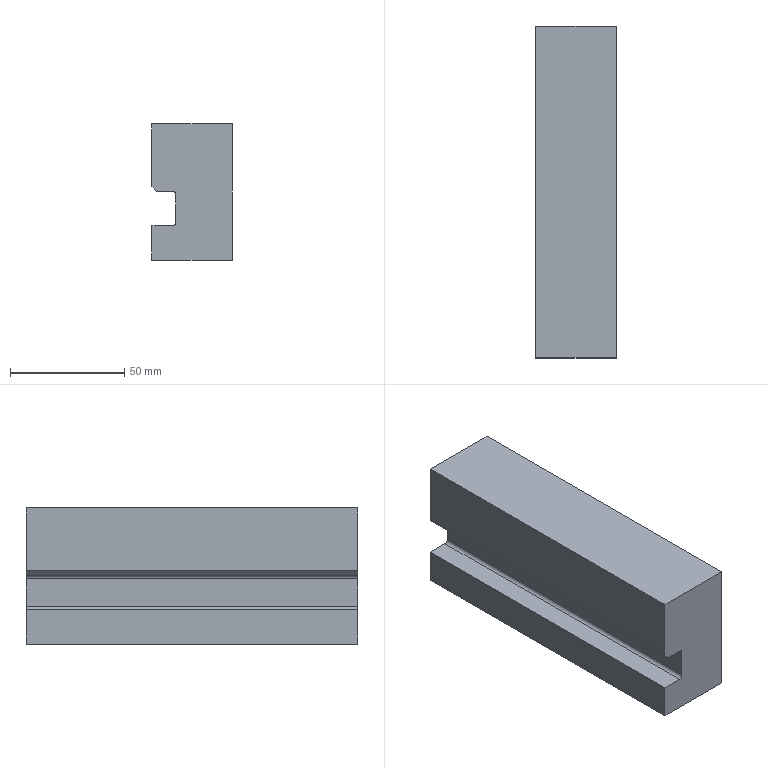Part | SolidWorks | features BaseBody 1 | 1 solid | 43 faces | box 35 x 145 x 59.5 mm | volume 272412 mm3 | plane 25 | cylinder 10 | cone 8 | commonest cylinder face diameters 8.5 x8 3 x2
STEP:
#1=CARTESIAN_POINT('',(214.249,235.,-60.));
#2=VERTEX_POINT('',#1);
#3=CARTESIAN_POINT('',(222.749,235.,-60.));
#4=VERTEX_POINT('',#3);
#5=CARTESIAN_POINT('',(218.499,235.,-60.));
#6=DIRECTION('',(0.,0.,-1.));
#7=DIRECTION('',(-1.,0.,0.));
#8=AXIS2_PLACEMENT_3D('',#5,#6,#7);
#9=CIRCLE('',#8,4.25);
#10=EDGE_CURVE('',#2,#4,#9,.T.);
#11=ORIENTED_EDGE('',*,*,#10,.T.);
#12=CARTESIAN_POINT('',(222.749,235.,-32.));
#13=VERTEX_POINT('',#12);
#14=CARTESIAN_POINT('',(222.749,235.,-60.));
#15=DIRECTION('',(0.,0.,1.));
#16=VECTOR('',#15,1000.);
#17=LINE('',#14,#16);
#18=EDGE_CURVE('',#4,#13,#17,.T.);
#19=ORIENTED_EDGE('',*,*,#18,.T.);
#20=CARTESIAN_POINT('',(214.249,235.,-32.));
#21=VERTEX_POINT('',#20);
#22=CARTESIAN_POINT('',(218.499,235.,-32.));
#23=DIRECTION('',(0.,0.,-1.));
#24=DIRECTION('',(-1.,0.,0.));
#25=AXIS2_PLACEMENT_3D('',#22,#23,#24);
#26=CIRCLE('',#25,4.25);
#27=EDGE_CURVE('',#21,#13,#26,.T.);
#28=ORIENTED_EDGE('',*,*,#27,.F.);
#29=CARTESIAN_POINT('',(214.249,235.,-60.));
#30=DIRECTION('',(0.,0.,1.));
#31=VECTOR('',#30,1000.);
#32=LINE('',#29,#31);
#33=EDGE_CURVE('',#2,#21,#32,.T.);
#34=ORIENTED_EDGE('',*,*,#33,.F.);
#35=EDGE_LOOP('',(#11,#19,#28,#34));
#36=FACE_OUTER_BOUND('',#35,.T.);
#37=CARTESIAN_POINT('',(218.499,235.,-60.));
#38=DIRECTION('',(0.,0.,1.));
#39=DIRECTION('',(-1.,0.,0.));
#40=AXIS2_PLACEMENT_3D('',#37,#38,#39);
#41=CYLINDRICAL_SURFACE('',#40,4.25);
#42=ADVANCED_FACE('',(#36),#41,.F.);
#43=CARTESIAN_POINT('',(218.499,235.,-29.446));
#44=VERTEX_POINT('',#43);
#45=CARTESIAN_POINT('',(222.749,235.,-32.));
#46=DIRECTION('',(0.8572,0.,-0.515));
#47=VECTOR('',#46,1000.);
#48=LINE('',#45,#47);
#49=EDGE_CURVE('',#44,#13,#48,.T.);
#50=ORIENTED_EDGE('',*,*,#49,.F.);
#51=CARTESIAN_POINT('',(214.249,235.,-32.));
#52=DIRECTION('',(-0.8572,0.,-0.515));
#53=VECTOR('',#52,1000.);
#54=LINE('',#51,#53);
#55=EDGE_CURVE('',#44,#21,#54,.T.);
#56=ORIENTED_EDGE('',*,*,#55,.T.);
#57=ORIENTED_EDGE('',*,*,#27,.T.);
#58=EDGE_LOOP('',(#50,#56,#57));
#59=FACE_OUTER_BOUND('',#58,.T.);
#60=CARTESIAN_POINT('',(218.499,235.,-32.));
#61=DIRECTION('',(0.,0.,-1.));
#62=DIRECTION('',(1.,0.,0.));
#63=AXIS2_PLACEMENT_3D('',#60,#61,#62);
#64=CONICAL_SURFACE('',#63,4.25,1.03);
#65=ADVANCED_FACE('',(#59),#64,.F.);
#66=CARTESIAN_POINT('',(214.249,270.,-60.));
#67=VERTEX_POINT('',#66);
#68=CARTESIAN_POINT('',(222.749,270.,-60.));
#69=VERTEX_POINT('',#68);
#70=CARTESIAN_POINT('',(218.499,270.,-60.));
#71=DIRECTION('',(0.,0.,-1.));
#72=DIRECTION('',(-1.,0.,0.));
#73=AXIS2_PLACEMENT_3D('',#70,#71,#72);
#74=CIRCLE('',#73,4.25);
#75=EDGE_CURVE('',#67,#69,#74,.T.);
#76=ORIENTED_EDGE('',*,*,#75,.T.);
#77=CARTESIAN_POINT('',(222.749,270.,-32.));
#78=VERTEX_POINT('',#77);
#79=CARTESIAN_POINT('',(222.749,270.,-60.));
#80=DIRECTION('',(0.,0.,1.));
#81=VECTOR('',#80,1000.);
#82=LINE('',#79,#81);
#83=EDGE_CURVE('',#69,#78,#82,.T.);
#84=ORIENTED_EDGE('',*,*,#83,.T.);
#85=CARTESIAN_POINT('',(214.249,270.,-32.));
#86=VERTEX_POINT('',#85);
#87=CARTESIAN_POINT('',(218.499,270.,-32.));
#88=DIRECTION('',(0.,0.,-1.));
#89=DIRECTION('',(-1.,0.,0.));
#90=AXIS2_PLACEMENT_3D('',#87,#88,#89);
#91=CIRCLE('',#90,4.25);
#92=EDGE_CURVE('',#86,#78,#91,.T.);
#93=ORIENTED_EDGE('',*,*,#92,.F.);
#94=CARTESIAN_POINT('',(214.249,270.,-60.));
#95=DIRECTION('',(0.,0.,1.));
#96=VECTOR('',#95,1000.);
#97=LINE('',#94,#96);
#98=EDGE_CURVE('',#67,#86,#97,.T.);
#99=ORIENTED_EDGE('',*,*,#98,.F.);
#100=EDGE_LOOP('',(#76,#84,#93,#99));
#101=FACE_OUTER_BOUND('',#100,.T.);
#102=CARTESIAN_POINT('',(218.499,270.,-60.));
#103=DIRECTION('',(0.,0.,1.));
#104=DIRECTION('',(-1.,0.,0.));
#105=AXIS2_PLACEMENT_3D('',#102,#103,#104);
#106=CYLINDRICAL_SURFACE('',#105,4.25);
#107=ADVANCED_FACE('',(#101),#106,.F.);
#108=CARTESIAN_POINT('',(218.499,270.,-29.446));
#109=VERTEX_POINT('',#108);
#110=CARTESIAN_POINT('',(222.749,270.,-32.));
#111=DIRECTION('',(0.8572,0.,-0.515));
#112=VECTOR('',#111,1000.);
#113=LINE('',#110,#112);
#114=EDGE_CURVE('',#109,#78,#113,.T.);
#115=ORIENTED_EDGE('',*,*,#114,.F.);
#116=CARTESIAN_POINT('',(214.249,270.,-32.));
#117=DIRECTION('',(-0.8572,0.,-0.515));
#118=VECTOR('',#117,1000.);
#119=LINE('',#116,#118);
#120=EDGE_CURVE('',#109,#86,#119,.T.);
#121=ORIENTED_EDGE('',*,*,#120,.T.);
#122=ORIENTED_EDGE('',*,*,#92,.T.);
#123=EDGE_LOOP('',(#115,#121,#122));
#124=FACE_OUTER_BOUND('',#123,.T.);
#125=CARTESIAN_POINT('',(218.499,270.,-32.));
#126=DIRECTION('',(0.,0.,-1.));
#127=DIRECTION('',(1.,0.,0.));
#128=AXIS2_PLACEMENT_3D('',#125,#126,#127);
#129=CONICAL_SURFACE('',#128,4.25,1.03);
#130=ADVANCED_FACE('',(#124),#129,.F.);
#131=CARTESIAN_POINT('',(214.249,300.,-60.));
#132=VERTEX_POINT('',#131);
#133=CARTESIAN_POINT('',(222.749,300.,-60.));
#134=VERTEX_POINT('',#133);
#135=CARTESIAN_POINT('',(218.499,300.,-60.));
#136=DIRECTION('',(0.,0.,-1.));
#137=DIRECTION('',(-1.,0.,0.));
#138=AXIS2_PLACEMENT_3D('',#135,#136,#137);
#139=CIRCLE('',#138,4.25);
#140=EDGE_CURVE('',#132,#134,#139,.T.);
#141=ORIENTED_EDGE('',*,*,#140,.T.);
#142=CARTESIAN_POINT('',(222.749,300.,-32.));
#143=VERTEX_POINT('',#142);
#144=CARTESIAN_POINT('',(222.749,300.,-60.));
#145=DIRECTION('',(0.,0.,1.));
#146=VECTOR('',#145,1000.);
#147=LINE('',#144,#146);
#148=EDGE_CURVE('',#134,#143,#147,.T.);
#149=ORIENTED_EDGE('',*,*,#148,.T.);
#150=CARTESIAN_POINT('',(214.249,300.,-32.));
#151=VERTEX_POINT('',#150);
#152=CARTESIAN_POINT('',(218.499,300.,-32.));
#153=DIRECTION('',(0.,0.,-1.));
#154=DIRECTION('',(-1.,0.,0.));
#155=AXIS2_PLACEMENT_3D('',#152,#153,#154);
#156=CIRCLE('',#155,4.25);
#157=EDGE_CURVE('',#151,#143,#156,.T.);
#158=ORIENTED_EDGE('',*,*,#157,.F.);
#159=CARTESIAN_POINT('',(214.249,300.,-60.));
#160=DIRECTION('',(0.,0.,1.));
#161=VECTOR('',#160,1000.);
#162=LINE('',#159,#161);
#163=EDGE_CURVE('',#132,#151,#162,.T.);
#164=ORIENTED_EDGE('',*,*,#163,.F.);
#165=EDGE_LOOP('',(#141,#149,#158,#164));
#166=FACE_OUTER_BOUND('',#165,.T.);
#167=CARTESIAN_POINT('',(218.499,300.,-60.));
#168=DIRECTION('',(0.,0.,1.));
#169=DIRECTION('',(-1.,0.,0.));
#170=AXIS2_PLACEMENT_3D('',#167,#168,#169);
#171=CYLINDRICAL_SURFACE('',#170,4.25);
#172=ADVANCED_FACE('',(#166),#171,.F.);
#173=CARTESIAN_POINT('',(218.499,300.,-29.446));
#174=VERTEX_POINT('',#173);
#175=CARTESIAN_POINT('',(222.749,300.,-32.));
#176=DIRECTION('',(0.8572,0.,-0.515));
#177=VECTOR('',#176,1000.);
#178=LINE('',#175,#177);
#179=EDGE_CURVE('',#174,#143,#178,.T.);
#180=ORIENTED_EDGE('',*,*,#179,.F.);
#181=CARTESIAN_POINT('',(214.249,300.,-32.));
#182=DIRECTION('',(-0.8572,0.,-0.515));
#183=VECTOR('',#182,1000.);
#184=LINE('',#181,#183);
#185=EDGE_CURVE('',#174,#151,#184,.T.);
#186=ORIENTED_EDGE('',*,*,#185,.T.);
#187=ORIENTED_EDGE('',*,*,#157,.T.);
#188=EDGE_LOOP('',(#180,#186,#187));
#189=FACE_OUTER_BOUND('',#188,.T.);
#190=CARTESIAN_POINT('',(218.499,300.,-32.));
#191=DIRECTION('',(0.,0.,-1.));
#192=DIRECTION('',(1.,0.,0.));
#193=AXIS2_PLACEMENT_3D('',#190,#191,#192);
#194=CONICAL_SURFACE('',#193,4.25,1.03);
#195=ADVANCED_FACE('',(#189),#194,.F.);
#196=CARTESIAN_POINT('',(214.249,335.,-60.));
#197=VERTEX_POINT('',#196);
#198=CARTESIAN_POINT('',(222.749,335.,-60.));
#199=VERTEX_POINT('',#198);
#200=CARTESIAN_POINT('',(218.499,335.,-60.));
#201=DIRECTION('',(0.,0.,-1.));
#202=DIRECTION('',(-1.,0.,0.));
#203=AXIS2_PLACEMENT_3D('',#200,#201,#202);
#204=CIRCLE('',#203,4.25);
#205=EDGE_CURVE('',#197,#199,#204,.T.);
#206=ORIENTED_EDGE('',*,*,#205,.T.);
#207=CARTESIAN_POINT('',(222.749,335.,-32.));
#208=VERTEX_POINT('',#207);
#209=CARTESIAN_POINT('',(222.749,335.,-60.));
#210=DIRECTION('',(0.,0.,1.));
#211=VECTOR('',#210,1000.);
#212=LINE('',#209,#211);
#213=EDGE_CURVE('',#199,#208,#212,.T.);
#214=ORIENTED_EDGE('',*,*,#213,.T.);
#215=CARTESIAN_POINT('',(214.249,335.,-32.));
#216=VERTEX_POINT('',#215);
#217=CARTESIAN_POINT('',(218.499,335.,-32.));
#218=DIRECTION('',(0.,0.,-1.));
#219=DIRECTION('',(-1.,0.,0.));
#220=AXIS2_PLACEMENT_3D('',#217,#218,#219);
#221=CIRCLE('',#220,4.25);
#222=EDGE_CURVE('',#216,#208,#221,.T.);
#223=ORIENTED_EDGE('',*,*,#222,.F.);
#224=CARTESIAN_POINT('',(214.249,335.,-60.));
#225=DIRECTION('',(0.,0.,1.));
#226=VECTOR('',#225,1000.);
#227=LINE('',#224,#226);
#228=EDGE_CURVE('',#197,#216,#227,.T.);
#229=ORIENTED_EDGE('',*,*,#228,.F.);
#230=EDGE_LOOP('',(#206,#214,#223,#229));
#231=FACE_OUTER_BOUND('',#230,.T.);
#232=CARTESIAN_POINT('',(218.499,335.,-60.));
#233=DIRECTION('',(0.,0.,1.));
#234=DIRECTION('',(-1.,0.,0.));
#235=AXIS2_PLACEMENT_3D('',#232,#233,#234);
#236=CYLINDRICAL_SURFACE('',#235,4.25);
#237=ADVANCED_FACE('',(#231),#236,.F.);
#238=CARTESIAN_POINT('',(218.499,335.,-29.446));
#239=VERTEX_POINT('',#238);
#240=CARTESIAN_POINT('',(222.749,335.,-32.));
#241=DIRECTION('',(0.8572,0.,-0.515));
#242=VECTOR('',#241,1000.);
#243=LINE('',#240,#242);
#244=EDGE_CURVE('',#239,#208,#243,.T.);
#245=ORIENTED_EDGE('',*,*,#244,.F.);
#246=CARTESIAN_POINT('',(214.249,335.,-32.));
#247=DIRECTION('',(-0.8572,0.,-0.515));
#248=VECTOR('',#247,1000.);
#249=LINE('',#246,#248);
#250=EDGE_CURVE('',#239,#216,#249,.T.);
#251=ORIENTED_EDGE('',*,*,#250,.T.);
#252=ORIENTED_EDGE('',*,*,#222,.T.);
#253=EDGE_LOOP('',(#245,#251,#252));
#254=FACE_OUTER_BOUND('',#253,.T.);
#255=CARTESIAN_POINT('',(218.499,335.,-32.));
#256=DIRECTION('',(0.,0.,-1.));
#257=DIRECTION('',(1.,0.,0.));
#258=AXIS2_PLACEMENT_3D('',#255,#256,#257);
#259=CONICAL_SURFACE('',#258,4.25,1.03);
#260=ADVANCED_FACE('',(#254),#259,.F.);
#261=ORIENTED_EDGE('',*,*,#10,.F.);
#262=CARTESIAN_POINT('',(218.499,235.,-60.));
#263=DIRECTION('',(0.,0.,-1.));
#264=DIRECTION('',(-1.,0.,0.));
#265=AXIS2_PLACEMENT_3D('',#262,#263,#264);
#266=CIRCLE('',#265,4.25);
#267=EDGE_CURVE('',#4,#2,#266,.T.);
#268=ORIENTED_EDGE('',*,*,#267,.F.);
#269=EDGE_LOOP('',(#261,#268));
#270=FACE_BOUND('',#269,.T.);
#271=ORIENTED_EDGE('',*,*,#75,.F.);
#272=CARTESIAN_POINT('',(218.499,270.,-60.));
#273=DIRECTION('',(0.,0.,-1.));
#274=DIRECTION('',(-1.,0.,0.));
#275=AXIS2_PLACEMENT_3D('',#272,#273,#274);
#276=CIRCLE('',#275,4.25);
#277=EDGE_CURVE('',#69,#67,#276,.T.);
#278=ORIENTED_EDGE('',*,*,#277,.F.);
#279=EDGE_LOOP('',(#271,#278));
#280=FACE_BOUND('',#279,.T.);
#281=ORIENTED_EDGE('',*,*,#140,.F.);
#282=CARTESIAN_POINT('',(218.499,300.,-60.));
#283=DIRECTION('',(0.,0.,-1.));
#284=DIRECTION('',(-1.,0.,0.));
#285=AXIS2_PLACEMENT_3D('',#282,#283,#284);
#286=CIRCLE('',#285,4.25);
#287=EDGE_CURVE('',#134,#132,#286,.T.);
#288=ORIENTED_EDGE('',*,*,#287,.F.);
#289=EDGE_LOOP('',(#281,#288));
#290=FACE_BOUND('',#289,.T.);
#291=ORIENTED_EDGE('',*,*,#205,.F.);
#292=CARTESIAN_POINT('',(218.499,335.,-60.));
#293=DIRECTION('',(0.,0.,-1.));
#294=DIRECTION('',(-1.,0.,0.));
#295=AXIS2_PLACEMENT_3D('',#292,#293,#294);
#296=CIRCLE('',#295,4.25);
#297=EDGE_CURVE('',#199,#197,#296,.T.);
#298=ORIENTED_EDGE('',*,*,#297,.F.);
#299=EDGE_LOOP('',(#291,#298));
#300=FACE_BOUND('',#299,.T.);
#301=CARTESIAN_POINT('',(196.,205.,-60.));
#302=VERTEX_POINT('',#301);
#303=CARTESIAN_POINT('',(196.,350.,-60.));
#304=VERTEX_POINT('',#303);
#305=CARTESIAN_POINT('',(196.,280.,-60.));
#306=DIRECTION('',(0.,1.,0.));
#307=VECTOR('',#306,1000.);
#308=LINE('',#305,#307);
#309=EDGE_CURVE('',#302,#304,#308,.T.);
#310=ORIENTED_EDGE('',*,*,#309,.T.);
#311=CARTESIAN_POINT('',(231.,350.,-60.));
#312=VERTEX_POINT('',#311);
#313=CARTESIAN_POINT('',(-265.,350.,-60.));
#314=DIRECTION('',(1.,0.,0.));
#315=VECTOR('',#314,1000.);
#316=LINE('',#313,#315);
#317=EDGE_CURVE('',#304,#312,#316,.T.);
#318=ORIENTED_EDGE('',*,*,#317,.T.);
#319=CARTESIAN_POINT('',(231.,205.,-60.));
#320=VERTEX_POINT('',#319);
#321=CARTESIAN_POINT('',(231.,280.,-60.));
#322=DIRECTION('',(0.,-1.,0.));
#323=VECTOR('',#322,1000.);
#324=LINE('',#321,#323);
#325=EDGE_CURVE('',#312,#320,#324,.T.);
#326=ORIENTED_EDGE('',*,*,#325,.T.);
#327=CARTESIAN_POINT('',(213.5,205.,-60.));
#328=DIRECTION('',(-1.,0.,0.));
#329=VECTOR('',#328,1000.);
#330=LINE('',#327,#329);
#331=EDGE_CURVE('',#320,#302,#330,.T.);
#332=ORIENTED_EDGE('',*,*,#331,.T.);
#333=EDGE_LOOP('',(#310,#318,#326,#332));
#334=FACE_OUTER_BOUND('',#333,.T.);
#335=CARTESIAN_POINT('',(225.677,215.697,-60.));
#336=VERTEX_POINT('',#335);
#337=CARTESIAN_POINT('',(225.677,219.697,-60.));
#338=VERTEX_POINT('',#337);
#339=CARTESIAN_POINT('',(225.677,215.697,-60.));
#340=DIRECTION('',(0.,1.,0.));
#341=VECTOR('',#340,1000.);
#342=LINE('',#339,#341);
#343=EDGE_CURVE('',#336,#338,#342,.T.);
#344=ORIENTED_EDGE('',*,*,#343,.F.);
#345=CARTESIAN_POINT('',(220.677,215.697,-60.));
#346=VERTEX_POINT('',#345);
#347=CARTESIAN_POINT('',(225.677,215.697,-60.));
#348=DIRECTION('',(-1.,0.,0.));
#349=VECTOR('',#348,1000.);
#350=LINE('',#347,#349);
#351=EDGE_CURVE('',#336,#346,#350,.T.);
#352=ORIENTED_EDGE('',*,*,#351,.T.);
#353=CARTESIAN_POINT('',(220.677,210.697,-60.));
#354=VERTEX_POINT('',#353);
#355=CARTESIAN_POINT('',(220.677,210.697,-60.));
#356=DIRECTION('',(0.,1.,0.));
#357=VECTOR('',#356,1000.);
#358=LINE('',#355,#357);
#359=EDGE_CURVE('',#354,#346,#358,.T.);
#360=ORIENTED_EDGE('',*,*,#359,.F.);
#361=CARTESIAN_POINT('',(216.677,210.697,-60.));
#362=VERTEX_POINT('',#361);
#363=CARTESIAN_POINT('',(220.677,210.697,-60.));
#364=DIRECTION('',(-1.,0.,0.));
#365=VECTOR('',#364,1000.);
#366=LINE('',#363,#365);
#367=EDGE_CURVE('',#354,#362,#366,.T.);
#368=ORIENTED_EDGE('',*,*,#367,.T.);
#369=CARTESIAN_POINT('',(216.677,209.697,-60.));
#370=VERTEX_POINT('',#369);
#371=CARTESIAN_POINT('',(216.677,210.697,-60.));
#372=DIRECTION('',(0.,-1.,0.));
#373=VECTOR('',#372,1000.);
#374=LINE('',#371,#373);
#375=EDGE_CURVE('',#362,#370,#374,.T.);
#376=ORIENTED_EDGE('',*,*,#375,.T.);
#377=CARTESIAN_POINT('',(226.677,209.697,-60.));
#378=VERTEX_POINT('',#377);
#379=CARTESIAN_POINT('',(226.677,209.697,-60.));
#380=DIRECTION('',(-1.,0.,0.));
#381=VECTOR('',#380,1000.);
#382=LINE('',#379,#381);
#383=EDGE_CURVE('',#378,#370,#382,.T.);
#384=ORIENTED_EDGE('',*,*,#383,.F.);
#385=CARTESIAN_POINT('',(226.677,219.697,-60.));
#386=VERTEX_POINT('',#385);
#387=CARTESIAN_POINT('',(226.677,209.697,-60.));
#388=DIRECTION('',(0.,1.,0.));
#389=VECTOR('',#388,1000.);
#390=LINE('',#387,#389);
#391=EDGE_CURVE('',#378,#386,#390,.T.);
#392=ORIENTED_EDGE('',*,*,#391,.T.);
#393=CARTESIAN_POINT('',(226.677,219.697,-60.));
#394=DIRECTION('',(-1.,0.,0.));
#395=VECTOR('',#394,1000.);
#396=LINE('',#393,#395);
#397=EDGE_CURVE('',#386,#338,#396,.T.);
#398=ORIENTED_EDGE('',*,*,#397,.T.);
#399=EDGE_LOOP('',(#344,#352,#360,#368,#376,#384,#392,#398));
#400=FACE_BOUND('',#399,.T.);
#401=CARTESIAN_POINT('',(-265.,308.35,-60.));
#402=DIRECTION('',(0.,0.,1.));
#403=DIRECTION('',(-1.,0.,0.));
#404=AXIS2_PLACEMENT_3D('',#401,#402,#403);
#405=PLANE('',#404);
#406=ADVANCED_FACE('',(#270,#280,#290,#300,#334,#400),#405,.F.);
#407=CARTESIAN_POINT('',(205.,205.,-30.));
#408=VERTEX_POINT('',#407);
#409=CARTESIAN_POINT('',(198.,205.,-30.));
#410=VERTEX_POINT('',#409);
#411=CARTESIAN_POINT('',(203.5,205.,-30.));
#412=DIRECTION('',(-1.,0.,0.));
#413=VECTOR('',#412,1000.);
#414=LINE('',#411,#413);
#415=EDGE_CURVE('',#408,#410,#414,.T.);
#416=ORIENTED_EDGE('',*,*,#415,.F.);
#417=CARTESIAN_POINT('',(206.5,205.,-31.5));
#418=VERTEX_POINT('',#417);
#419=CARTESIAN_POINT('',(205.,205.,-31.5));
#420=DIRECTION('',(0.,-1.,0.));
#421=DIRECTION('',(0.,0.,-1.));
#422=AXIS2_PLACEMENT_3D('',#419,#420,#421);
#423=CIRCLE('',#422,1.5);
#424=EDGE_CURVE('',#418,#408,#423,.T.);
#425=ORIENTED_EDGE('',*,*,#424,.F.);
#426=CARTESIAN_POINT('',(206.5,205.,-43.5));
#427=VERTEX_POINT('',#426);
#428=CARTESIAN_POINT('',(206.5,205.,-45.));
#429=DIRECTION('',(0.,0.,1.));
#430=VECTOR('',#429,1000.);
#431=LINE('',#428,#430);
#432=EDGE_CURVE('',#427,#418,#431,.T.);
#433=ORIENTED_EDGE('',*,*,#432,.F.);
#434=CARTESIAN_POINT('',(205.,205.,-45.));
#435=VERTEX_POINT('',#434);
#436=CARTESIAN_POINT('',(205.,205.,-43.5));
#437=DIRECTION('',(0.,-1.,0.));
#438=DIRECTION('',(0.,0.,-1.));
#439=AXIS2_PLACEMENT_3D('',#436,#437,#438);
#440=CIRCLE('',#439,1.5);
#441=EDGE_CURVE('',#435,#427,#440,.T.);
#442=ORIENTED_EDGE('',*,*,#441,.F.);
#443=CARTESIAN_POINT('',(196.,205.,-45.));
#444=VERTEX_POINT('',#443);
#445=CARTESIAN_POINT('',(213.5,205.,-45.));
#446=DIRECTION('',(-1.,0.,0.));
#447=VECTOR('',#446,1000.);
#448=LINE('',#445,#447);
#449=EDGE_CURVE('',#435,#444,#448,.T.);
#450=ORIENTED_EDGE('',*,*,#449,.T.);
#451=CARTESIAN_POINT('',(196.,205.,-60.));
#452=DIRECTION('',(0.,0.,1.));
#453=VECTOR('',#452,1000.);
#454=LINE('',#451,#453);
#455=EDGE_CURVE('',#302,#444,#454,.T.);
#456=ORIENTED_EDGE('',*,*,#455,.F.);
#457=ORIENTED_EDGE('',*,*,#331,.F.);
#458=CARTESIAN_POINT('',(231.,205.,-0.5));
#459=VERTEX_POINT('',#458);
#460=CARTESIAN_POINT('',(231.,205.,-38.));
#461=DIRECTION('',(0.,0.,1.));
#462=VECTOR('',#461,1000.);
#463=LINE('',#460,#462);
#464=EDGE_CURVE('',#320,#459,#463,.T.);
#465=ORIENTED_EDGE('',*,*,#464,.T.);
#466=CARTESIAN_POINT('',(196.,205.,-0.5));
#467=VERTEX_POINT('',#466);
#468=CARTESIAN_POINT('',(213.5,205.,-0.5));
#469=DIRECTION('',(1.,0.,0.));
#470=VECTOR('',#469,1000.);
#471=LINE('',#468,#470);
#472=EDGE_CURVE('',#467,#459,#471,.T.);
#473=ORIENTED_EDGE('',*,*,#472,.F.);
#474=CARTESIAN_POINT('',(196.,205.,-28.));
#475=VERTEX_POINT('',#474);
#476=CARTESIAN_POINT('',(196.,205.,-38.));
#477=DIRECTION('',(0.,0.,1.));
#478=VECTOR('',#477,1000.);
#479=LINE('',#476,#478);
#480=EDGE_CURVE('',#475,#467,#479,.T.);
#481=ORIENTED_EDGE('',*,*,#480,.F.);
#482=CARTESIAN_POINT('',(209.75,205.,-41.75));
#483=DIRECTION('',(-0.7071,0.,0.7071));
#484=VECTOR('',#483,1000.);
#485=LINE('',#482,#484);
#486=EDGE_CURVE('',#410,#475,#485,.T.);
#487=ORIENTED_EDGE('',*,*,#486,.F.);
#488=EDGE_LOOP('',(#416,#425,#433,#442,#450,#456,#457,#465,#473,#481,#487));
#489=FACE_OUTER_BOUND('',#488,.T.);
#490=CARTESIAN_POINT('',(213.5,205.,-38.));
#491=DIRECTION('',(0.,-1.,0.));
#492=DIRECTION('',(0.,0.,-1.));
#493=AXIS2_PLACEMENT_3D('',#490,#491,#492);
#494=PLANE('',#493);
#495=ADVANCED_FACE('',(#489),#494,.T.);
#496=ORIENTED_EDGE('',*,*,#472,.T.);
#497=CARTESIAN_POINT('',(231.,350.,-0.5));
#498=VERTEX_POINT('',#497);
#499=CARTESIAN_POINT('',(231.,280.,-0.5));
#500=DIRECTION('',(0.,1.,0.));
#501=VECTOR('',#500,1000.);
#502=LINE('',#499,#501);
#503=EDGE_CURVE('',#459,#498,#502,.T.);
#504=ORIENTED_EDGE('',*,*,#503,.T.);
#505=CARTESIAN_POINT('',(196.,350.,-0.5));
#506=VERTEX_POINT('',#505);
#507=CARTESIAN_POINT('',(213.5,350.,-0.5));
#508=DIRECTION('',(-1.,0.,0.));
#509=VECTOR('',#508,1000.);
#510=LINE('',#507,#509);
#511=EDGE_CURVE('',#498,#506,#510,.T.);
#512=ORIENTED_EDGE('',*,*,#511,.T.);
#513=CARTESIAN_POINT('',(196.,280.,-0.5));
#514=DIRECTION('',(0.,-1.,0.));
#515=VECTOR('',#514,1000.);
#516=LINE('',#513,#515);
#517=EDGE_CURVE('',#506,#467,#516,.T.);
#518=ORIENTED_EDGE('',*,*,#517,.T.);
#519=EDGE_LOOP('',(#496,#504,#512,#518));
#520=FACE_OUTER_BOUND('',#519,.T.);
#521=CARTESIAN_POINT('',(213.5,280.,-0.5));
#522=DIRECTION('',(0.,0.,1.));
#523=DIRECTION('',(-1.,0.,0.));
#524=AXIS2_PLACEMENT_3D('',#521,#522,#523);
#525=PLANE('',#524);
#526=ADVANCED_FACE('',(#520),#525,.T.);
#527=ORIENTED_EDGE('',*,*,#464,.F.);
#528=ORIENTED_EDGE('',*,*,#325,.F.);
#529=CARTESIAN_POINT('',(231.,350.,-38.));
#530=DIRECTION('',(0.,0.,1.));
#531=VECTOR('',#530,1000.);
#532=LINE('',#529,#531);
#533=EDGE_CURVE('',#312,#498,#532,.T.);
#534=ORIENTED_EDGE('',*,*,#533,.T.);
#535=ORIENTED_EDGE('',*,*,#503,.F.);
#536=EDGE_LOOP('',(#527,#528,#534,#535));
#537=FACE_OUTER_BOUND('',#536,.T.);
#538=CARTESIAN_POINT('',(231.,280.,-38.));
#539=DIRECTION('',(1.,0.,0.));
#540=DIRECTION('',(0.,0.,1.));
#541=AXIS2_PLACEMENT_3D('',#538,#539,#540);
#542=PLANE('',#541);
#543=ADVANCED_FACE('',(#537),#542,.T.);
#544=CARTESIAN_POINT('',(196.,350.,-28.));
#545=VERTEX_POINT('',#544);
#546=CARTESIAN_POINT('',(196.,350.,-135.5));
#547=DIRECTION('',(0.,0.,1.));
#548=VECTOR('',#547,1000.);
#549=LINE('',#546,#548);
#550=EDGE_CURVE('',#545,#506,#549,.T.);
#551=ORIENTED_EDGE('',*,*,#550,.T.);
#552=ORIENTED_EDGE('',*,*,#511,.F.);
#553=ORIENTED_EDGE('',*,*,#533,.F.);
#554=ORIENTED_EDGE('',*,*,#317,.F.);
#555=CARTESIAN_POINT('',(196.,350.,-45.));
#556=VERTEX_POINT('',#555);
#557=CARTESIAN_POINT('',(196.,350.,-135.5));
#558=DIRECTION('',(0.,0.,1.));
#559=VECTOR('',#558,1000.);
#560=LINE('',#557,#559);
#561=EDGE_CURVE('',#304,#556,#560,.T.);
#562=ORIENTED_EDGE('',*,*,#561,.T.);
#563=CARTESIAN_POINT('',(205.,350.,-45.));
#564=VERTEX_POINT('',#563);
#565=CARTESIAN_POINT('',(-265.,350.,-45.));
#566=DIRECTION('',(1.,0.,0.));
#567=VECTOR('',#566,1000.);
#568=LINE('',#565,#567);
#569=EDGE_CURVE('',#556,#564,#568,.T.);
#570=ORIENTED_EDGE('',*,*,#569,.T.);
#571=CARTESIAN_POINT('',(206.5,350.,-43.5));
#572=VERTEX_POINT('',#571);
#573=CARTESIAN_POINT('',(205.,350.,-43.5));
#574=DIRECTION('',(0.,1.,0.));
#575=DIRECTION('',(0.,0.,-1.));
#576=AXIS2_PLACEMENT_3D('',#573,#574,#575);
#577=CIRCLE('',#576,1.5);
#578=EDGE_CURVE('',#572,#564,#577,.T.);
#579=ORIENTED_EDGE('',*,*,#578,.F.);
#580=CARTESIAN_POINT('',(206.5,350.,-31.5));
#581=VERTEX_POINT('',#580);
#582=CARTESIAN_POINT('',(206.5,350.,-45.));
#583=DIRECTION('',(0.,0.,1.));
#584=VECTOR('',#583,1000.);
#585=LINE('',#582,#584);
#586=EDGE_CURVE('',#572,#581,#585,.T.);
#587=ORIENTED_EDGE('',*,*,#586,.T.);
#588=CARTESIAN_POINT('',(205.,350.,-30.));
#589=VERTEX_POINT('',#588);
#590=CARTESIAN_POINT('',(205.,350.,-31.5));
#591=DIRECTION('',(0.,1.,0.));
#592=DIRECTION('',(0.,0.,-1.));
#593=AXIS2_PLACEMENT_3D('',#590,#591,#592);
#594=CIRCLE('',#593,1.5);
#595=EDGE_CURVE('',#589,#581,#594,.T.);
#596=ORIENTED_EDGE('',*,*,#595,.F.);
#597=CARTESIAN_POINT('',(198.,350.,-30.));
#598=VERTEX_POINT('',#597);
#599=CARTESIAN_POINT('',(256.,350.,-30.));
#600=DIRECTION('',(1.,0.,0.));
#601=VECTOR('',#600,1000.);
#602=LINE('',#599,#601);
#603=EDGE_CURVE('',#598,#589,#602,.T.);
#604=ORIENTED_EDGE('',*,*,#603,.F.);
#605=CARTESIAN_POINT('',(196.,350.,-28.));
#606=DIRECTION('',(0.7071,0.,-0.7071));
#607=VECTOR('',#606,1000.);
#608=LINE('',#605,#607);
#609=EDGE_CURVE('',#545,#598,#608,.T.);
#610=ORIENTED_EDGE('',*,*,#609,.F.);
#611=EDGE_LOOP('',(#551,#552,#553,#554,#562,#570,#579,#587,#596,#604,#610));
#612=FACE_OUTER_BOUND('',#611,.T.);
#613=CARTESIAN_POINT('',(256.,350.,-135.5));
#614=DIRECTION('',(0.,-1.,0.));
#615=DIRECTION('',(0.,0.,-1.));
#616=AXIS2_PLACEMENT_3D('',#613,#614,#615);
#617=PLANE('',#616);
#618=ADVANCED_FACE('',(#612),#617,.F.);
#619=ORIENTED_EDGE('',*,*,#480,.T.);
#620=ORIENTED_EDGE('',*,*,#517,.F.);
#621=ORIENTED_EDGE('',*,*,#550,.F.);
#622=CARTESIAN_POINT('',(196.,355.,-28.));
#623=DIRECTION('',(0.,1.,0.));
#624=VECTOR('',#623,1000.);
#625=LINE('',#622,#624);
#626=EDGE_CURVE('',#475,#545,#625,.T.);
#627=ORIENTED_EDGE('',*,*,#626,.F.);
#628=EDGE_LOOP('',(#619,#620,#621,#627));
#629=FACE_OUTER_BOUND('',#628,.T.);
#630=CARTESIAN_POINT('',(196.,280.,-38.));
#631=DIRECTION('',(-1.,0.,0.));
#632=DIRECTION('',(0.,0.,-1.));
#633=AXIS2_PLACEMENT_3D('',#630,#631,#632);
#634=PLANE('',#633);
#635=ADVANCED_FACE('',(#629),#634,.T.);
#636=ORIENTED_EDGE('',*,*,#603,.T.);
#637=CARTESIAN_POINT('',(205.,355.,-30.));
#638=DIRECTION('',(0.,1.,0.));
#639=VECTOR('',#638,1000.);
#640=LINE('',#637,#639);
#641=EDGE_CURVE('',#408,#589,#640,.T.);
#642=ORIENTED_EDGE('',*,*,#641,.F.);
#643=ORIENTED_EDGE('',*,*,#415,.T.);
#644=CARTESIAN_POINT('',(198.,205.,-30.));
#645=DIRECTION('',(0.,-1.,0.));
#646=VECTOR('',#645,1000.);
#647=LINE('',#644,#646);
#648=EDGE_CURVE('',#598,#410,#647,.T.);
#649=ORIENTED_EDGE('',*,*,#648,.F.);
#650=EDGE_LOOP('',(#636,#642,#643,#649));
#651=FACE_OUTER_BOUND('',#650,.T.);
#652=CARTESIAN_POINT('',(203.5,256.675,-30.));
#653=DIRECTION('',(0.,0.,1.));
#654=DIRECTION('',(1.,0.,0.));
#655=AXIS2_PLACEMENT_3D('',#652,#653,#654);
#656=PLANE('',#655);
#657=ADVANCED_FACE('',(#651),#656,.F.);
#658=ORIENTED_EDGE('',*,*,#432,.T.);
#659=CARTESIAN_POINT('',(206.5,205.,-31.5));
#660=DIRECTION('',(0.,-1.,0.));
#661=VECTOR('',#660,1000.);
#662=LINE('',#659,#661);
#663=EDGE_CURVE('',#581,#418,#662,.T.);
#664=ORIENTED_EDGE('',*,*,#663,.F.);
#665=ORIENTED_EDGE('',*,*,#586,.F.);
#666=CARTESIAN_POINT('',(206.5,355.,-43.5));
#667=DIRECTION('',(0.,1.,0.));
#668=VECTOR('',#667,1000.);
#669=LINE('',#666,#668);
#670=EDGE_CURVE('',#427,#572,#669,.T.);
#671=ORIENTED_EDGE('',*,*,#670,.F.);
#672=EDGE_LOOP('',(#658,#664,#665,#671));
#673=FACE_OUTER_BOUND('',#672,.T.);
#674=CARTESIAN_POINT('',(206.5,256.675,-45.));
#675=DIRECTION('',(1.,0.,0.));
#676=DIRECTION('',(0.,0.,-1.));
#677=AXIS2_PLACEMENT_3D('',#674,#675,#676);
#678=PLANE('',#677);
#679=ADVANCED_FACE('',(#673),#678,.F.);
#680=CARTESIAN_POINT('',(196.,280.,-45.));
#681=DIRECTION('',(0.,1.,0.));
#682=VECTOR('',#681,1000.);
#683=LINE('',#680,#682);
#684=EDGE_CURVE('',#444,#556,#683,.T.);
#685=ORIENTED_EDGE('',*,*,#684,.T.);
#686=ORIENTED_EDGE('',*,*,#561,.F.);
#687=ORIENTED_EDGE('',*,*,#309,.F.);
#688=ORIENTED_EDGE('',*,*,#455,.T.);
#689=EDGE_LOOP('',(#685,#686,#687,#688));
#690=FACE_OUTER_BOUND('',#689,.T.);
#691=CARTESIAN_POINT('',(196.,280.,-38.));
#692=DIRECTION('',(-1.,0.,0.));
#693=DIRECTION('',(0.,0.,-1.));
#694=AXIS2_PLACEMENT_3D('',#691,#692,#693);
#695=PLANE('',#694);
#696=ADVANCED_FACE('',(#690),#695,.T.);
#697=ORIENTED_EDGE('',*,*,#569,.F.);
#698=ORIENTED_EDGE('',*,*,#684,.F.);
#699=ORIENTED_EDGE('',*,*,#449,.F.);
#700=CARTESIAN_POINT('',(205.,205.,-45.));
#701=DIRECTION('',(0.,-1.,0.));
#702=VECTOR('',#701,1000.);
#703=LINE('',#700,#702);
#704=EDGE_CURVE('',#564,#435,#703,.T.);
#705=ORIENTED_EDGE('',*,*,#704,.F.);
#706=EDGE_LOOP('',(#697,#698,#699,#705));
#707=FACE_OUTER_BOUND('',#706,.T.);
#708=CARTESIAN_POINT('',(-265.,308.35,-45.));
#709=DIRECTION('',(0.,0.,1.));
#710=DIRECTION('',(-1.,0.,0.));
#711=AXIS2_PLACEMENT_3D('',#708,#709,#710);
#712=PLANE('',#711);
#713=ADVANCED_FACE('',(#707),#712,.T.);
#714=ORIENTED_EDGE('',*,*,#441,.T.);
#715=ORIENTED_EDGE('',*,*,#670,.T.);
#716=ORIENTED_EDGE('',*,*,#578,.T.);
#717=ORIENTED_EDGE('',*,*,#704,.T.);
#718=EDGE_LOOP('',(#714,#715,#716,#717));
#719=FACE_OUTER_BOUND('',#718,.T.);
#720=CARTESIAN_POINT('',(205.,256.675,-43.5));
#721=DIRECTION('',(0.,1.,0.));
#722=DIRECTION('',(0.,0.,1.));
#723=AXIS2_PLACEMENT_3D('',#720,#721,#722);
#724=CYLINDRICAL_SURFACE('',#723,1.5);
#725=ADVANCED_FACE('',(#719),#724,.F.);
#726=ORIENTED_EDGE('',*,*,#595,.T.);
#727=ORIENTED_EDGE('',*,*,#663,.T.);
#728=ORIENTED_EDGE('',*,*,#424,.T.);
#729=ORIENTED_EDGE('',*,*,#641,.T.);
#730=EDGE_LOOP('',(#726,#727,#728,#729));
#731=FACE_OUTER_BOUND('',#730,.T.);
#732=CARTESIAN_POINT('',(205.,256.675,-31.5));
#733=DIRECTION('',(0.,1.,0.));
#734=DIRECTION('',(0.,0.,1.));
#735=AXIS2_PLACEMENT_3D('',#732,#733,#734);
#736=CYLINDRICAL_SURFACE('',#735,1.5);
#737=ADVANCED_FACE('',(#731),#736,.F.);
#738=ORIENTED_EDGE('',*,*,#486,.T.);
#739=ORIENTED_EDGE('',*,*,#626,.T.);
#740=ORIENTED_EDGE('',*,*,#609,.T.);
#741=ORIENTED_EDGE('',*,*,#648,.T.);
#742=EDGE_LOOP('',(#738,#739,#740,#741));
#743=FACE_OUTER_BOUND('',#742,.T.);
#744=CARTESIAN_POINT('',(196.,280.,-28.));
#745=DIRECTION('',(-0.7071,0.,-0.7071));
#746=DIRECTION('',(0.7071,0.,-0.7071));
#747=AXIS2_PLACEMENT_3D('',#744,#745,#746);
#748=PLANE('',#747);
#749=ADVANCED_FACE('',(#743),#748,.T.);
#750=ORIENTED_EDGE('',*,*,#250,.F.);
#751=ORIENTED_EDGE('',*,*,#244,.T.);
#752=CARTESIAN_POINT('',(218.499,335.,-32.));
#753=DIRECTION('',(0.,0.,-1.));
#754=DIRECTION('',(-1.,0.,0.));
#755=AXIS2_PLACEMENT_3D('',#752,#753,#754);
#756=CIRCLE('',#755,4.25);
#757=EDGE_CURVE('',#208,#216,#756,.T.);
#758=ORIENTED_EDGE('',*,*,#757,.T.);
#759=EDGE_LOOP('',(#750,#751,#758));
#760=FACE_OUTER_BOUND('',#759,.T.);
#761=CARTESIAN_POINT('',(218.499,335.,-32.));
#762=DIRECTION('',(0.,0.,-1.));
#763=DIRECTION('',(1.,0.,0.));
#764=AXIS2_PLACEMENT_3D('',#761,#762,#763);
#765=CONICAL_SURFACE('',#764,4.25,1.03);
#766=ADVANCED_FACE('',(#760),#765,.F.);
#767=ORIENTED_EDGE('',*,*,#213,.F.);
#768=ORIENTED_EDGE('',*,*,#297,.T.);
#769=ORIENTED_EDGE('',*,*,#228,.T.);
#770=ORIENTED_EDGE('',*,*,#757,.F.);
#771=EDGE_LOOP('',(#767,#768,#769,#770));
#772=FACE_OUTER_BOUND('',#771,.T.);
#773=CARTESIAN_POINT('',(218.499,335.,-60.));
#774=DIRECTION('',(0.,0.,1.));
#775=DIRECTION('',(-1.,0.,0.));
#776=AXIS2_PLACEMENT_3D('',#773,#774,#775);
#777=CYLINDRICAL_SURFACE('',#776,4.25);
#778=ADVANCED_FACE('',(#772),#777,.F.);
#779=ORIENTED_EDGE('',*,*,#185,.F.);
#780=ORIENTED_EDGE('',*,*,#179,.T.);
#781=CARTESIAN_POINT('',(218.499,300.,-32.));
#782=DIRECTION('',(0.,0.,-1.));
#783=DIRECTION('',(-1.,0.,0.));
#784=AXIS2_PLACEMENT_3D('',#781,#782,#783);
#785=CIRCLE('',#784,4.25);
#786=EDGE_CURVE('',#143,#151,#785,.T.);
#787=ORIENTED_EDGE('',*,*,#786,.T.);
#788=EDGE_LOOP('',(#779,#780,#787));
#789=FACE_OUTER_BOUND('',#788,.T.);
#790=CARTESIAN_POINT('',(218.499,300.,-32.));
#791=DIRECTION('',(0.,0.,-1.));
#792=DIRECTION('',(1.,0.,0.));
#793=AXIS2_PLACEMENT_3D('',#790,#791,#792);
#794=CONICAL_SURFACE('',#793,4.25,1.03);
#795=ADVANCED_FACE('',(#789),#794,.F.);
#796=ORIENTED_EDGE('',*,*,#148,.F.);
#797=ORIENTED_EDGE('',*,*,#287,.T.);
#798=ORIENTED_EDGE('',*,*,#163,.T.);
#799=ORIENTED_EDGE('',*,*,#786,.F.);
#800=EDGE_LOOP('',(#796,#797,#798,#799));
#801=FACE_OUTER_BOUND('',#800,.T.);
#802=CARTESIAN_POINT('',(218.499,300.,-60.));
#803=DIRECTION('',(0.,0.,1.));
#804=DIRECTION('',(-1.,0.,0.));
#805=AXIS2_PLACEMENT_3D('',#802,#803,#804);
#806=CYLINDRICAL_SURFACE('',#805,4.25);
#807=ADVANCED_FACE('',(#801),#806,.F.);
#808=ORIENTED_EDGE('',*,*,#120,.F.);
#809=ORIENTED_EDGE('',*,*,#114,.T.);
#810=CARTESIAN_POINT('',(218.499,270.,-32.));
#811=DIRECTION('',(0.,0.,-1.));
#812=DIRECTION('',(-1.,0.,0.));
#813=AXIS2_PLACEMENT_3D('',#810,#811,#812);
#814=CIRCLE('',#813,4.25);
#815=EDGE_CURVE('',#78,#86,#814,.T.);
#816=ORIENTED_EDGE('',*,*,#815,.T.);
#817=EDGE_LOOP('',(#808,#809,#816));
#818=FACE_OUTER_BOUND('',#817,.T.);
#819=CARTESIAN_POINT('',(218.499,270.,-32.));
#820=DIRECTION('',(0.,0.,-1.));
#821=DIRECTION('',(1.,0.,0.));
#822=AXIS2_PLACEMENT_3D('',#819,#820,#821);
#823=CONICAL_SURFACE('',#822,4.25,1.03);
#824=ADVANCED_FACE('',(#818),#823,.F.);
#825=ORIENTED_EDGE('',*,*,#83,.F.);
#826=ORIENTED_EDGE('',*,*,#277,.T.);
#827=ORIENTED_EDGE('',*,*,#98,.T.);
#828=ORIENTED_EDGE('',*,*,#815,.F.);
#829=EDGE_LOOP('',(#825,#826,#827,#828));
#830=FACE_OUTER_BOUND('',#829,.T.);
#831=CARTESIAN_POINT('',(218.499,270.,-60.));
#832=DIRECTION('',(0.,0.,1.));
#833=DIRECTION('',(-1.,0.,0.));
#834=AXIS2_PLACEMENT_3D('',#831,#832,#833);
#835=CYLINDRICAL_SURFACE('',#834,4.25);
#836=ADVANCED_FACE('',(#830),#835,.F.);
#837=ORIENTED_EDGE('',*,*,#55,.F.);
#838=ORIENTED_EDGE('',*,*,#49,.T.);
#839=CARTESIAN_POINT('',(218.499,235.,-32.));
#840=DIRECTION('',(0.,0.,-1.));
#841=DIRECTION('',(-1.,0.,0.));
#842=AXIS2_PLACEMENT_3D('',#839,#840,#841);
#843=CIRCLE('',#842,4.25);
#844=EDGE_CURVE('',#13,#21,#843,.T.);
#845=ORIENTED_EDGE('',*,*,#844,.T.);
#846=EDGE_LOOP('',(#837,#838,#845));
#847=FACE_OUTER_BOUND('',#846,.T.);
#848=CARTESIAN_POINT('',(218.499,235.,-32.));
#849=DIRECTION('',(0.,0.,-1.));
#850=DIRECTION('',(1.,0.,0.));
#851=AXIS2_PLACEMENT_3D('',#848,#849,#850);
#852=CONICAL_SURFACE('',#851,4.25,1.03);
#853=ADVANCED_FACE('',(#847),#852,.F.);
#854=ORIENTED_EDGE('',*,*,#18,.F.);
#855=ORIENTED_EDGE('',*,*,#267,.T.);
#856=ORIENTED_EDGE('',*,*,#33,.T.);
#857=ORIENTED_EDGE('',*,*,#844,.F.);
#858=EDGE_LOOP('',(#854,#855,#856,#857));
#859=FACE_OUTER_BOUND('',#858,.T.);
#860=CARTESIAN_POINT('',(218.499,235.,-60.));
#861=DIRECTION('',(0.,0.,1.));
#862=DIRECTION('',(-1.,0.,0.));
#863=AXIS2_PLACEMENT_3D('',#860,#861,#862);
#864=CYLINDRICAL_SURFACE('',#863,4.25);
#865=ADVANCED_FACE('',(#859),#864,.F.);
#866=CARTESIAN_POINT('',(225.677,210.697,-60.));
#867=VERTEX_POINT('',#866);
#868=CARTESIAN_POINT('',(225.677,214.697,-60.));
#869=VERTEX_POINT('',#868);
#870=CARTESIAN_POINT('',(225.677,210.697,-60.));
#871=DIRECTION('',(0.,1.,0.));
#872=VECTOR('',#871,1000.);
#873=LINE('',#870,#872);
#874=EDGE_CURVE('',#867,#869,#873,.T.);
#875=ORIENTED_EDGE('',*,*,#874,.T.);
#876=CARTESIAN_POINT('',(225.677,214.697,-59.5));
#877=VERTEX_POINT('',#876);
#878=CARTESIAN_POINT('',(225.677,214.697,-59.5));
#879=DIRECTION('',(0.,0.,-1.));
#880=VECTOR('',#879,1000.);
#881=LINE('',#878,#880);
#882=EDGE_CURVE('',#877,#869,#881,.T.);
#883=ORIENTED_EDGE('',*,*,#882,.F.);
#884=CARTESIAN_POINT('',(225.677,210.697,-59.5));
#885=VERTEX_POINT('',#884);
#886=CARTESIAN_POINT('',(225.677,210.697,-59.5));
#887=DIRECTION('',(0.,1.,0.));
#888=VECTOR('',#887,1000.);
#889=LINE('',#886,#888);
#890=EDGE_CURVE('',#885,#877,#889,.T.);
#891=ORIENTED_EDGE('',*,*,#890,.F.);
#892=CARTESIAN_POINT('',(225.677,210.697,-59.5));
#893=DIRECTION('',(0.,0.,-1.));
#894=VECTOR('',#893,1000.);
#895=LINE('',#892,#894);
#896=EDGE_CURVE('',#885,#867,#895,.T.);
#897=ORIENTED_EDGE('',*,*,#896,.T.);
#898=EDGE_LOOP('',(#875,#883,#891,#897));
#899=FACE_OUTER_BOUND('',#898,.T.);
#900=CARTESIAN_POINT('',(225.677,210.697,-59.5));
#901=DIRECTION('',(1.,0.,0.));
#902=DIRECTION('',(0.,0.,1.));
#903=AXIS2_PLACEMENT_3D('',#900,#901,#902);
#904=PLANE('',#903);
#905=ADVANCED_FACE('',(#899),#904,.T.);
#906=CARTESIAN_POINT('',(221.677,210.697,-60.));
#907=VERTEX_POINT('',#906);
#908=CARTESIAN_POINT('',(225.677,210.697,-60.));
#909=DIRECTION('',(-1.,0.,0.));
#910=VECTOR('',#909,1000.);
#911=LINE('',#908,#910);
#912=EDGE_CURVE('',#867,#907,#911,.T.);
#913=ORIENTED_EDGE('',*,*,#912,.F.);
#914=ORIENTED_EDGE('',*,*,#896,.F.);
#915=CARTESIAN_POINT('',(221.677,210.697,-59.5));
#916=VERTEX_POINT('',#915);
#917=CARTESIAN_POINT('',(225.677,210.697,-59.5));
#918=DIRECTION('',(-1.,0.,0.));
#919=VECTOR('',#918,1000.);
#920=LINE('',#917,#919);
#921=EDGE_CURVE('',#885,#916,#920,.T.);
#922=ORIENTED_EDGE('',*,*,#921,.T.);
#923=CARTESIAN_POINT('',(221.677,210.697,-59.5));
#924=DIRECTION('',(0.,0.,-1.));
#925=VECTOR('',#924,1000.);
#926=LINE('',#923,#925);
#927=EDGE_CURVE('',#916,#907,#926,.T.);
#928=ORIENTED_EDGE('',*,*,#927,.T.);
#929=EDGE_LOOP('',(#913,#914,#922,#928));
#930=FACE_OUTER_BOUND('',#929,.T.);
#931=CARTESIAN_POINT('',(225.677,210.697,-59.5));
#932=DIRECTION('',(0.,1.,0.));
#933=DIRECTION('',(0.,0.,1.));
#934=AXIS2_PLACEMENT_3D('',#931,#932,#933);
#935=PLANE('',#934);
#936=ADVANCED_FACE('',(#930),#935,.F.);
#937=CARTESIAN_POINT('',(221.677,214.697,-60.));
#938=VERTEX_POINT('',#937);
#939=CARTESIAN_POINT('',(221.677,210.697,-60.));
#940=DIRECTION('',(0.,1.,0.));
#941=VECTOR('',#940,1000.);
#942=LINE('',#939,#941);
#943=EDGE_CURVE('',#907,#938,#942,.T.);
#944=ORIENTED_EDGE('',*,*,#943,.F.);
#945=ORIENTED_EDGE('',*,*,#927,.F.);
#946=CARTESIAN_POINT('',(221.677,214.697,-59.5));
#947=VERTEX_POINT('',#946);
#948=CARTESIAN_POINT('',(221.677,210.697,-59.5));
#949=DIRECTION('',(0.,1.,0.));
#950=VECTOR('',#949,1000.);
#951=LINE('',#948,#950);
#952=EDGE_CURVE('',#916,#947,#951,.T.);
#953=ORIENTED_EDGE('',*,*,#952,.T.);
#954=CARTESIAN_POINT('',(221.677,214.697,-59.5));
#955=DIRECTION('',(0.,0.,-1.));
#956=VECTOR('',#955,1000.);
#957=LINE('',#954,#956);
#958=EDGE_CURVE('',#947,#938,#957,.T.);
#959=ORIENTED_EDGE('',*,*,#958,.T.);
#960=EDGE_LOOP('',(#944,#945,#953,#959));
#961=FACE_OUTER_BOUND('',#960,.T.);
#962=CARTESIAN_POINT('',(221.677,210.697,-59.5));
#963=DIRECTION('',(1.,0.,0.));
#964=DIRECTION('',(0.,0.,1.));
#965=AXIS2_PLACEMENT_3D('',#962,#963,#964);
#966=PLANE('',#965);
#967=ADVANCED_FACE('',(#961),#966,.F.);
#968=ORIENTED_EDGE('',*,*,#351,.F.);
#969=CARTESIAN_POINT('',(225.677,215.697,-59.5));
#970=VERTEX_POINT('',#969);
#971=CARTESIAN_POINT('',(225.677,215.697,-59.5));
#972=DIRECTION('',(0.,0.,-1.));
#973=VECTOR('',#972,1000.);
#974=LINE('',#971,#973);
#975=EDGE_CURVE('',#970,#336,#974,.T.);
#976=ORIENTED_EDGE('',*,*,#975,.F.);
#977=CARTESIAN_POINT('',(220.677,215.697,-59.5));
#978=VERTEX_POINT('',#977);
#979=CARTESIAN_POINT('',(225.677,215.697,-59.5));
#980=DIRECTION('',(-1.,0.,0.));
#981=VECTOR('',#980,1000.);
#982=LINE('',#979,#981);
#983=EDGE_CURVE('',#970,#978,#982,.T.);
#984=ORIENTED_EDGE('',*,*,#983,.T.);
#985=CARTESIAN_POINT('',(220.677,215.697,-59.5));
#986=DIRECTION('',(0.,0.,-1.));
#987=VECTOR('',#986,1000.);
#988=LINE('',#985,#987);
#989=EDGE_CURVE('',#978,#346,#988,.T.);
#990=ORIENTED_EDGE('',*,*,#989,.T.);
#991=EDGE_LOOP('',(#968,#976,#984,#990));
#992=FACE_OUTER_BOUND('',#991,.T.);
#993=CARTESIAN_POINT('',(225.677,215.697,-59.5));
#994=DIRECTION('',(0.,1.,0.));
#995=DIRECTION('',(0.,0.,1.));
#996=AXIS2_PLACEMENT_3D('',#993,#994,#995);
#997=PLANE('',#996);
#998=ADVANCED_FACE('',(#992),#997,.F.);
#999=ORIENTED_EDGE('',*,*,#359,.T.);
#1000=ORIENTED_EDGE('',*,*,#989,.F.);
#1001=CARTESIAN_POINT('',(220.677,210.697,-59.5));
#1002=VERTEX_POINT('',#1001);
#1003=CARTESIAN_POINT('',(220.677,210.697,-59.5));
#1004=DIRECTION('',(0.,1.,0.));
#1005=VECTOR('',#1004,1000.);
#1006=LINE('',#1003,#1005);
#1007=EDGE_CURVE('',#1002,#978,#1006,.T.);
#1008=ORIENTED_EDGE('',*,*,#1007,.F.);
#1009=CARTESIAN_POINT('',(220.677,210.697,-59.5));
#1010=DIRECTION('',(0.,0.,-1.));
#1011=VECTOR('',#1010,1000.);
#1012=LINE('',#1009,#1011);
#1013=EDGE_CURVE('',#1002,#354,#1012,.T.);
#1014=ORIENTED_EDGE('',*,*,#1013,.T.);
#1015=EDGE_LOOP('',(#999,#1000,#1008,#1014));
#1016=FACE_OUTER_BOUND('',#1015,.T.);
#1017=CARTESIAN_POINT('',(220.677,210.697,-59.5));
#1018=DIRECTION('',(1.,0.,0.));
#1019=DIRECTION('',(0.,0.,1.));
#1020=AXIS2_PLACEMENT_3D('',#1017,#1018,#1019);
#1021=PLANE('',#1020);
#1022=ADVANCED_FACE('',(#1016),#1021,.T.);
#1023=ORIENTED_EDGE('',*,*,#367,.F.);
#1024=ORIENTED_EDGE('',*,*,#1013,.F.);
#1025=CARTESIAN_POINT('',(216.677,210.697,-59.5));
#1026=VERTEX_POINT('',#1025);
#1027=CARTESIAN_POINT('',(220.677,210.697,-59.5));
#1028=DIRECTION('',(-1.,0.,0.));
#1029=VECTOR('',#1028,1000.);
#1030=LINE('',#1027,#1029);
#1031=EDGE_CURVE('',#1002,#1026,#1030,.T.);
#1032=ORIENTED_EDGE('',*,*,#1031,.T.);
#1033=CARTESIAN_POINT('',(216.677,210.697,-59.5));
#1034=DIRECTION('',(0.,0.,-1.));
#1035=VECTOR('',#1034,1000.);
#1036=LINE('',#1033,#1035);
#1037=EDGE_CURVE('',#1026,#362,#1036,.T.);
#1038=ORIENTED_EDGE('',*,*,#1037,.T.);
#1039=EDGE_LOOP('',(#1023,#1024,#1032,#1038));
#1040=FACE_OUTER_BOUND('',#1039,.T.);
#1041=CARTESIAN_POINT('',(220.677,210.697,-59.5));
#1042=DIRECTION('',(0.,1.,0.));
#1043=DIRECTION('',(0.,0.,1.));
#1044=AXIS2_PLACEMENT_3D('',#1041,#1042,#1043);
#1045=PLANE('',#1044);
#1046=ADVANCED_FACE('',(#1040),#1045,.F.);
#1047=ORIENTED_EDGE('',*,*,#375,.F.);
#1048=ORIENTED_EDGE('',*,*,#1037,.F.);
#1049=CARTESIAN_POINT('',(216.677,209.697,-59.5));
#1050=VERTEX_POINT('',#1049);
#1051=CARTESIAN_POINT('',(216.677,210.697,-59.5));
#1052=DIRECTION('',(0.,-1.,0.));
#1053=VECTOR('',#1052,1000.);
#1054=LINE('',#1051,#1053);
#1055=EDGE_CURVE('',#1026,#1050,#1054,.T.);
#1056=ORIENTED_EDGE('',*,*,#1055,.T.);
#1057=CARTESIAN_POINT('',(216.677,209.697,-59.5));
#1058=DIRECTION('',(0.,0.,-1.));
#1059=VECTOR('',#1058,1000.);
#1060=LINE('',#1057,#1059);
#1061=EDGE_CURVE('',#1050,#370,#1060,.T.);
#1062=ORIENTED_EDGE('',*,*,#1061,.T.);
#1063=EDGE_LOOP('',(#1047,#1048,#1056,#1062));
#1064=FACE_OUTER_BOUND('',#1063,.T.);
#1065=CARTESIAN_POINT('',(216.677,210.697,-59.5));
#1066=DIRECTION('',(-1.,0.,0.));
#1067=DIRECTION('',(0.,0.,-1.));
#1068=AXIS2_PLACEMENT_3D('',#1065,#1066,#1067);
#1069=PLANE('',#1068);
#1070=ADVANCED_FACE('',(#1064),#1069,.F.);
#1071=ORIENTED_EDGE('',*,*,#383,.T.);
#1072=ORIENTED_EDGE('',*,*,#1061,.F.);
#1073=CARTESIAN_POINT('',(226.677,209.697,-59.5));
#1074=VERTEX_POINT('',#1073);
#1075=CARTESIAN_POINT('',(226.677,209.697,-59.5));
#1076=DIRECTION('',(-1.,0.,0.));
#1077=VECTOR('',#1076,1000.);
#1078=LINE('',#1075,#1077);
#1079=EDGE_CURVE('',#1074,#1050,#1078,.T.);
#1080=ORIENTED_EDGE('',*,*,#1079,.F.);
#1081=CARTESIAN_POINT('',(226.677,209.697,-59.5));
#1082=DIRECTION('',(0.,0.,-1.));
#1083=VECTOR('',#1082,1000.);
#1084=LINE('',#1081,#1083);
#1085=EDGE_CURVE('',#1074,#378,#1084,.T.);
#1086=ORIENTED_EDGE('',*,*,#1085,.T.);
#1087=EDGE_LOOP('',(#1071,#1072,#1080,#1086));
#1088=FACE_OUTER_BOUND('',#1087,.T.);
#1089=CARTESIAN_POINT('',(226.677,209.697,-59.5));
#1090=DIRECTION('',(0.,1.,0.));
#1091=DIRECTION('',(0.,0.,1.));
#1092=AXIS2_PLACEMENT_3D('',#1089,#1090,#1091);
#1093=PLANE('',#1092);
#1094=ADVANCED_FACE('',(#1088),#1093,.T.);
#1095=ORIENTED_EDGE('',*,*,#391,.F.);
#1096=ORIENTED_EDGE('',*,*,#1085,.F.);
#1097=CARTESIAN_POINT('',(226.677,219.697,-59.5));
#1098=VERTEX_POINT('',#1097);
#1099=CARTESIAN_POINT('',(226.677,209.697,-59.5));
#1100=DIRECTION('',(0.,1.,0.));
#1101=VECTOR('',#1100,1000.);
#1102=LINE('',#1099,#1101);
#1103=EDGE_CURVE('',#1074,#1098,#1102,.T.);
#1104=ORIENTED_EDGE('',*,*,#1103,.T.);
#1105=CARTESIAN_POINT('',(226.677,219.697,-59.5));
#1106=DIRECTION('',(0.,0.,-1.));
#1107=VECTOR('',#1106,1000.);
#1108=LINE('',#1105,#1107);
#1109=EDGE_CURVE('',#1098,#386,#1108,.T.);
#1110=ORIENTED_EDGE('',*,*,#1109,.T.);
#1111=EDGE_LOOP('',(#1095,#1096,#1104,#1110));
#1112=FACE_OUTER_BOUND('',#1111,.T.);
#1113=CARTESIAN_POINT('',(226.677,209.697,-59.5));
#1114=DIRECTION('',(1.,0.,0.));
#1115=DIRECTION('',(0.,0.,1.));
#1116=AXIS2_PLACEMENT_3D('',#1113,#1114,#1115);
#1117=PLANE('',#1116);
#1118=ADVANCED_FACE('',(#1112),#1117,.F.);
#1119=ORIENTED_EDGE('',*,*,#397,.F.);
#1120=ORIENTED_EDGE('',*,*,#1109,.F.);
#1121=CARTESIAN_POINT('',(225.677,219.697,-59.5));
#1122=VERTEX_POINT('',#1121);
#1123=CARTESIAN_POINT('',(226.677,219.697,-59.5));
#1124=DIRECTION('',(-1.,0.,0.));
#1125=VECTOR('',#1124,1000.);
#1126=LINE('',#1123,#1125);
#1127=EDGE_CURVE('',#1098,#1122,#1126,.T.);
#1128=ORIENTED_EDGE('',*,*,#1127,.T.);
#1129=CARTESIAN_POINT('',(225.677,219.697,-59.5));
#1130=DIRECTION('',(0.,0.,-1.));
#1131=VECTOR('',#1130,1000.);
#1132=LINE('',#1129,#1131);
#1133=EDGE_CURVE('',#1122,#338,#1132,.T.);
#1134=ORIENTED_EDGE('',*,*,#1133,.T.);
#1135=EDGE_LOOP('',(#1119,#1120,#1128,#1134));
#1136=FACE_OUTER_BOUND('',#1135,.T.);
#1137=CARTESIAN_POINT('',(226.677,219.697,-59.5));
#1138=DIRECTION('',(0.,1.,0.));
#1139=DIRECTION('',(0.,0.,1.));
#1140=AXIS2_PLACEMENT_3D('',#1137,#1138,#1139);
#1141=PLANE('',#1140);
#1142=ADVANCED_FACE('',(#1136),#1141,.F.);
#1143=ORIENTED_EDGE('',*,*,#343,.T.);
#1144=ORIENTED_EDGE('',*,*,#1133,.F.);
#1145=CARTESIAN_POINT('',(225.677,215.697,-59.5));
#1146=DIRECTION('',(0.,1.,0.));
#1147=VECTOR('',#1146,1000.);
#1148=LINE('',#1145,#1147);
#1149=EDGE_CURVE('',#970,#1122,#1148,.T.);
#1150=ORIENTED_EDGE('',*,*,#1149,.F.);
#1151=ORIENTED_EDGE('',*,*,#975,.T.);
#1152=EDGE_LOOP('',(#1143,#1144,#1150,#1151));
#1153=FACE_OUTER_BOUND('',#1152,.T.);
#1154=CARTESIAN_POINT('',(225.677,215.697,-59.5));
#1155=DIRECTION('',(1.,0.,0.));
#1156=DIRECTION('',(0.,0.,1.));
#1157=AXIS2_PLACEMENT_3D('',#1154,#1155,#1156);
#1158=PLANE('',#1157);
#1159=ADVANCED_FACE('',(#1153),#1158,.T.);
#1160=CARTESIAN_POINT('',(225.677,214.697,-60.));
#1161=DIRECTION('',(-1.,0.,0.));
#1162=VECTOR('',#1161,1000.);
#1163=LINE('',#1160,#1162);
#1164=EDGE_CURVE('',#869,#938,#1163,.T.);
#1165=ORIENTED_EDGE('',*,*,#1164,.T.);
#1166=ORIENTED_EDGE('',*,*,#958,.F.);
#1167=CARTESIAN_POINT('',(225.677,214.697,-59.5));
#1168=DIRECTION('',(-1.,0.,0.));
#1169=VECTOR('',#1168,1000.);
#1170=LINE('',#1167,#1169);
#1171=EDGE_CURVE('',#877,#947,#1170,.T.);
#1172=ORIENTED_EDGE('',*,*,#1171,.F.);
#1173=ORIENTED_EDGE('',*,*,#882,.T.);
#1174=EDGE_LOOP('',(#1165,#1166,#1172,#1173));
#1175=FACE_OUTER_BOUND('',#1174,.T.);
#1176=CARTESIAN_POINT('',(225.677,214.697,-59.5));
#1177=DIRECTION('',(0.,1.,0.));
#1178=DIRECTION('',(0.,0.,1.));
#1179=AXIS2_PLACEMENT_3D('',#1176,#1177,#1178);
#1180=PLANE('',#1179);
#1181=ADVANCED_FACE('',(#1175),#1180,.T.);
#1182=ORIENTED_EDGE('',*,*,#983,.F.);
#1183=ORIENTED_EDGE('',*,*,#1149,.T.);
#1184=ORIENTED_EDGE('',*,*,#1127,.F.);
#1185=ORIENTED_EDGE('',*,*,#1103,.F.);
#1186=ORIENTED_EDGE('',*,*,#1079,.T.);
#1187=ORIENTED_EDGE('',*,*,#1055,.F.);
#1188=ORIENTED_EDGE('',*,*,#1031,.F.);
#1189=ORIENTED_EDGE('',*,*,#1007,.T.);
#1190=EDGE_LOOP('',(#1182,#1183,#1184,#1185,#1186,#1187,#1188,#1189));
#1191=FACE_OUTER_BOUND('',#1190,.T.);
#1192=ORIENTED_EDGE('',*,*,#890,.T.);
#1193=ORIENTED_EDGE('',*,*,#1171,.T.);
#1194=ORIENTED_EDGE('',*,*,#952,.F.);
#1195=ORIENTED_EDGE('',*,*,#921,.F.);
#1196=EDGE_LOOP('',(#1192,#1193,#1194,#1195));
#1197=FACE_BOUND('',#1196,.T.);
#1198=CARTESIAN_POINT('',(220.677,215.697,-59.5));
#1199=DIRECTION('',(0.,0.,1.));
#1200=DIRECTION('',(-1.,0.,0.));
#1201=AXIS2_PLACEMENT_3D('',#1198,#1199,#1200);
#1202=PLANE('',#1201);
#1203=ADVANCED_FACE('',(#1191,#1197),#1202,.F.);
#1204=ORIENTED_EDGE('',*,*,#874,.F.);
#1205=ORIENTED_EDGE('',*,*,#912,.T.);
#1206=ORIENTED_EDGE('',*,*,#943,.T.);
#1207=ORIENTED_EDGE('',*,*,#1164,.F.);
#1208=EDGE_LOOP('',(#1204,#1205,#1206,#1207));
#1209=FACE_OUTER_BOUND('',#1208,.T.);
#1210=CARTESIAN_POINT('',(-265.,308.35,-60.));
#1211=DIRECTION('',(0.,0.,1.));
#1212=DIRECTION('',(-1.,0.,0.));
#1213=AXIS2_PLACEMENT_3D('',#1210,#1211,#1212);
#1214=PLANE('',#1213);
#1215=ADVANCED_FACE('',(#1209),#1214,.F.);
#1216=CLOSED_SHELL('',(#42,#65,#107,#130,#172,#195,#237,#260,#406,#495,#526,#543,#618,#635,#657,#679,#696,#713,#725,#737,#749,#766,#778,#795,#807,#824,#836,#853,#865,#905,#936,#967,#998,#1022,#1046,#1070,#1094,#1118,#1142,#1159,#1181,#1203,#1215));
#1217=MANIFOLD_SOLID_BREP('',#1216);
#1218=CARTESIAN_POINT('',(0.,0.,0.));
#1219=DIRECTION('',(0.,0.,1.));
#1220=DIRECTION('',(1.,0.,0.));
#1221=AXIS2_PLACEMENT_3D('',#1218,#1219,#1220);
#1222=(LENGTH_UNIT()NAMED_UNIT(*)SI_UNIT(.MILLI.,.METRE.));
#1223=UNCERTAINTY_MEASURE_WITH_UNIT(LENGTH_MEASURE(0.00001),#1222,'','');
#1224=(NAMED_UNIT(*)PLANE_ANGLE_UNIT()SI_UNIT($,.RADIAN.));
#1225=(NAMED_UNIT(*)SI_UNIT($,.STERADIAN.)SOLID_ANGLE_UNIT());
#1226=(GEOMETRIC_REPRESENTATION_CONTEXT(3)GLOBAL_UNCERTAINTY_ASSIGNED_CONTEXT((#1223))GLOBAL_UNIT_ASSIGNED_CONTEXT((#1222,#1224,#1225))REPRESENTATION_CONTEXT('',''));
#1227=ADVANCED_BREP_SHAPE_REPRESENTATION('',(#1217,#1221),#1226);